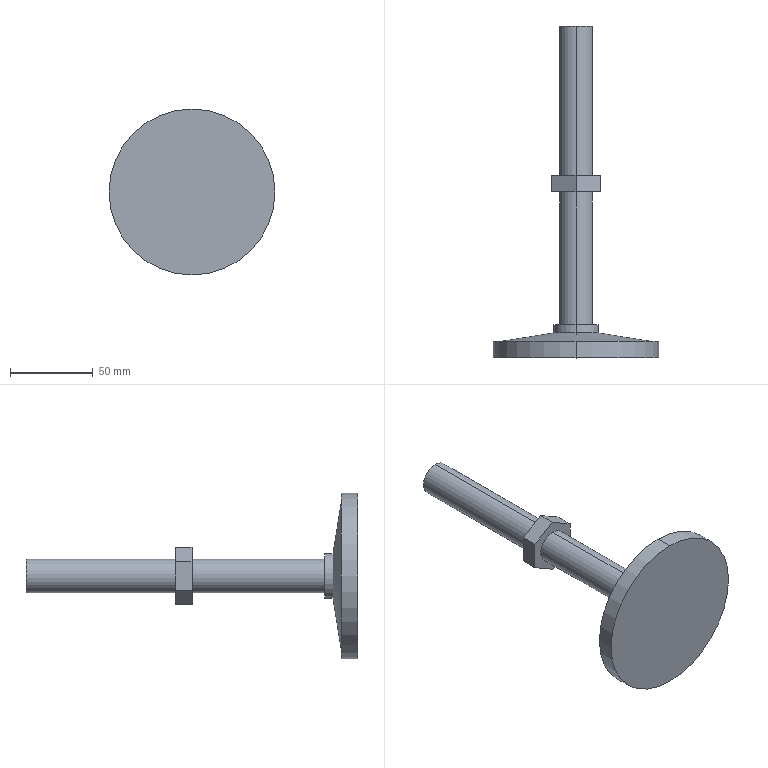Part | SolidWorks | features Boss 1, Revolution 1 | 1 solid | 22 faces | box 100 x 200 x 100 mm | volume 157266 mm3 | plane 12 | cylinder 8 | cone 2 | commonest cylinder face diameters 20 x4 26.809 x2 100 x2
STEP:
#1=CARTESIAN_POINT('',(0.,200.,-10.));
#2=VERTEX_POINT('',#1);
#3=CARTESIAN_POINT('',(0.,200.,10.));
#4=VERTEX_POINT('',#3);
#5=CARTESIAN_POINT('',(0.,200.,0.));
#6=DIRECTION('',(0.,-1.,0.));
#7=DIRECTION('',(0.,0.,-1.));
#8=AXIS2_PLACEMENT_3D('',#5,#6,#7);
#9=CIRCLE('',#8,10.);
#10=EDGE_CURVE('',#2,#4,#9,.T.);
#11=ORIENTED_EDGE('',*,*,#10,.T.);
#12=CARTESIAN_POINT('',(0.,110.,10.));
#13=VERTEX_POINT('',#12);
#14=CARTESIAN_POINT('',(0.,0.,10.));
#15=DIRECTION('',(0.,-1.,0.));
#16=VECTOR('',#15,1000.);
#17=LINE('',#14,#16);
#18=EDGE_CURVE('',#4,#13,#17,.T.);
#19=ORIENTED_EDGE('',*,*,#18,.T.);
#20=CARTESIAN_POINT('',(0.,110.,-10.));
#21=VERTEX_POINT('',#20);
#22=CARTESIAN_POINT('',(0.,110.,0.));
#23=DIRECTION('',(0.,1.,0.));
#24=DIRECTION('',(0.,0.,-1.));
#25=AXIS2_PLACEMENT_3D('',#22,#23,#24);
#26=CIRCLE('',#25,10.);
#27=EDGE_CURVE('',#13,#21,#26,.T.);
#28=ORIENTED_EDGE('',*,*,#27,.T.);
#29=CARTESIAN_POINT('',(0.,0.,-10.));
#30=DIRECTION('',(0.,-1.,0.));
#31=VECTOR('',#30,1000.);
#32=LINE('',#29,#31);
#33=EDGE_CURVE('',#2,#21,#32,.T.);
#34=ORIENTED_EDGE('',*,*,#33,.F.);
#35=EDGE_LOOP('',(#11,#19,#28,#34));
#36=FACE_OUTER_BOUND('',#35,.T.);
#37=CARTESIAN_POINT('',(0.,0.,0.));
#38=DIRECTION('',(0.,-1.,0.));
#39=DIRECTION('',(0.,0.,-1.));
#40=AXIS2_PLACEMENT_3D('',#37,#38,#39);
#41=CYLINDRICAL_SURFACE('',#40,10.);
#42=ADVANCED_FACE('',(#36),#41,.T.);
#43=CARTESIAN_POINT('',(0.,100.,10.));
#44=VERTEX_POINT('',#43);
#45=CARTESIAN_POINT('',(0.,100.,-10.));
#46=VERTEX_POINT('',#45);
#47=CARTESIAN_POINT('',(0.,100.,0.));
#48=DIRECTION('',(0.,1.,0.));
#49=DIRECTION('',(0.,0.,-1.));
#50=AXIS2_PLACEMENT_3D('',#47,#48,#49);
#51=CIRCLE('',#50,10.);
#52=EDGE_CURVE('',#44,#46,#51,.T.);
#53=ORIENTED_EDGE('',*,*,#52,.F.);
#54=CARTESIAN_POINT('',(0.,20.,10.));
#55=VERTEX_POINT('',#54);
#56=CARTESIAN_POINT('',(0.,0.,10.));
#57=DIRECTION('',(0.,-1.,0.));
#58=VECTOR('',#57,1000.);
#59=LINE('',#56,#58);
#60=EDGE_CURVE('',#44,#55,#59,.T.);
#61=ORIENTED_EDGE('',*,*,#60,.T.);
#62=CARTESIAN_POINT('',(0.,20.,-10.));
#63=VERTEX_POINT('',#62);
#64=CARTESIAN_POINT('',(0.,20.,0.));
#65=DIRECTION('',(0.,-1.,0.));
#66=DIRECTION('',(0.,0.,-1.));
#67=AXIS2_PLACEMENT_3D('',#64,#65,#66);
#68=CIRCLE('',#67,10.);
#69=EDGE_CURVE('',#63,#55,#68,.T.);
#70=ORIENTED_EDGE('',*,*,#69,.F.);
#71=CARTESIAN_POINT('',(0.,0.,-10.));
#72=DIRECTION('',(0.,-1.,0.));
#73=VECTOR('',#72,1000.);
#74=LINE('',#71,#73);
#75=EDGE_CURVE('',#46,#63,#74,.T.);
#76=ORIENTED_EDGE('',*,*,#75,.F.);
#77=EDGE_LOOP('',(#53,#61,#70,#76));
#78=FACE_OUTER_BOUND('',#77,.T.);
#79=CARTESIAN_POINT('',(0.,0.,0.));
#80=DIRECTION('',(0.,-1.,0.));
#81=DIRECTION('',(0.,0.,-1.));
#82=AXIS2_PLACEMENT_3D('',#79,#80,#81);
#83=CYLINDRICAL_SURFACE('',#82,10.);
#84=ADVANCED_FACE('',(#78),#83,.T.);
#85=CARTESIAN_POINT('',(0.,20.,-13.405));
#86=VERTEX_POINT('',#85);
#87=CARTESIAN_POINT('',(0.,20.,13.405));
#88=VERTEX_POINT('',#87);
#89=CARTESIAN_POINT('',(0.,20.,0.));
#90=DIRECTION('',(0.,-1.,0.));
#91=DIRECTION('',(0.,0.,-1.));
#92=AXIS2_PLACEMENT_3D('',#89,#90,#91);
#93=CIRCLE('',#92,13.405);
#94=EDGE_CURVE('',#86,#88,#93,.T.);
#95=ORIENTED_EDGE('',*,*,#94,.T.);
#96=CARTESIAN_POINT('',(0.,15.,13.405));
#97=VERTEX_POINT('',#96);
#98=CARTESIAN_POINT('',(0.,0.,13.405));
#99=DIRECTION('',(0.,-1.,0.));
#100=VECTOR('',#99,1000.);
#101=LINE('',#98,#100);
#102=EDGE_CURVE('',#88,#97,#101,.T.);
#103=ORIENTED_EDGE('',*,*,#102,.T.);
#104=CARTESIAN_POINT('',(0.,15.,-13.405));
#105=VERTEX_POINT('',#104);
#106=CARTESIAN_POINT('',(0.,15.,0.));
#107=DIRECTION('',(0.,-1.,0.));
#108=DIRECTION('',(0.,0.,-1.));
#109=AXIS2_PLACEMENT_3D('',#106,#107,#108);
#110=CIRCLE('',#109,13.405);
#111=EDGE_CURVE('',#105,#97,#110,.T.);
#112=ORIENTED_EDGE('',*,*,#111,.F.);
#113=CARTESIAN_POINT('',(0.,0.,-13.405));
#114=DIRECTION('',(0.,-1.,0.));
#115=VECTOR('',#114,1000.);
#116=LINE('',#113,#115);
#117=EDGE_CURVE('',#86,#105,#116,.T.);
#118=ORIENTED_EDGE('',*,*,#117,.F.);
#119=EDGE_LOOP('',(#95,#103,#112,#118));
#120=FACE_OUTER_BOUND('',#119,.T.);
#121=CARTESIAN_POINT('',(0.,0.,0.));
#122=DIRECTION('',(0.,-1.,0.));
#123=DIRECTION('',(0.,0.,-1.));
#124=AXIS2_PLACEMENT_3D('',#121,#122,#123);
#125=CYLINDRICAL_SURFACE('',#124,13.405);
#126=ADVANCED_FACE('',(#120),#125,.T.);
#127=ORIENTED_EDGE('',*,*,#111,.T.);
#128=CARTESIAN_POINT('',(0.,10.,45.));
#129=VERTEX_POINT('',#128);
#130=CARTESIAN_POINT('',(0.,10.,45.));
#131=DIRECTION('',(0.,-0.1563,0.9877));
#132=VECTOR('',#131,1000.);
#133=LINE('',#130,#132);
#134=EDGE_CURVE('',#97,#129,#133,.T.);
#135=ORIENTED_EDGE('',*,*,#134,.T.);
#136=CARTESIAN_POINT('',(0.,10.,-45.));
#137=VERTEX_POINT('',#136);
#138=CARTESIAN_POINT('',(0.,10.,0.));
#139=DIRECTION('',(0.,-1.,0.));
#140=DIRECTION('',(0.,0.,-1.));
#141=AXIS2_PLACEMENT_3D('',#138,#139,#140);
#142=CIRCLE('',#141,45.);
#143=EDGE_CURVE('',#137,#129,#142,.T.);
#144=ORIENTED_EDGE('',*,*,#143,.F.);
#145=CARTESIAN_POINT('',(0.,10.,-45.));
#146=DIRECTION('',(0.,-0.1563,-0.9877));
#147=VECTOR('',#146,1000.);
#148=LINE('',#145,#147);
#149=EDGE_CURVE('',#105,#137,#148,.T.);
#150=ORIENTED_EDGE('',*,*,#149,.F.);
#151=EDGE_LOOP('',(#127,#135,#144,#150));
#152=FACE_OUTER_BOUND('',#151,.T.);
#153=CARTESIAN_POINT('',(0.,10.,0.));
#154=DIRECTION('',(0.,-1.,0.));
#155=DIRECTION('',(0.,0.,-1.));
#156=AXIS2_PLACEMENT_3D('',#153,#154,#155);
#157=CONICAL_SURFACE('',#156,45.,1.414);
#158=ADVANCED_FACE('',(#152),#157,.T.);
#159=CARTESIAN_POINT('',(0.,10.,-50.));
#160=VERTEX_POINT('',#159);
#161=CARTESIAN_POINT('',(0.,10.,50.));
#162=VERTEX_POINT('',#161);
#163=CARTESIAN_POINT('',(0.,10.,0.));
#164=DIRECTION('',(0.,-1.,0.));
#165=DIRECTION('',(0.,0.,-1.));
#166=AXIS2_PLACEMENT_3D('',#163,#164,#165);
#167=CIRCLE('',#166,50.);
#168=EDGE_CURVE('',#160,#162,#167,.T.);
#169=ORIENTED_EDGE('',*,*,#168,.T.);
#170=CARTESIAN_POINT('',(0.,0.,50.));
#171=VERTEX_POINT('',#170);
#172=CARTESIAN_POINT('',(0.,0.,50.));
#173=DIRECTION('',(0.,-1.,0.));
#174=VECTOR('',#173,1000.);
#175=LINE('',#172,#174);
#176=EDGE_CURVE('',#162,#171,#175,.T.);
#177=ORIENTED_EDGE('',*,*,#176,.T.);
#178=CARTESIAN_POINT('',(0.,0.,-50.));
#179=VERTEX_POINT('',#178);
#180=CARTESIAN_POINT('',(0.,0.,0.));
#181=DIRECTION('',(0.,-1.,0.));
#182=DIRECTION('',(0.,0.,-1.));
#183=AXIS2_PLACEMENT_3D('',#180,#181,#182);
#184=CIRCLE('',#183,50.);
#185=EDGE_CURVE('',#179,#171,#184,.T.);
#186=ORIENTED_EDGE('',*,*,#185,.F.);
#187=CARTESIAN_POINT('',(0.,0.,-50.));
#188=DIRECTION('',(0.,-1.,0.));
#189=VECTOR('',#188,1000.);
#190=LINE('',#187,#189);
#191=EDGE_CURVE('',#160,#179,#190,.T.);
#192=ORIENTED_EDGE('',*,*,#191,.F.);
#193=EDGE_LOOP('',(#169,#177,#186,#192));
#194=FACE_OUTER_BOUND('',#193,.T.);
#195=CARTESIAN_POINT('',(0.,0.,0.));
#196=DIRECTION('',(0.,-1.,0.));
#197=DIRECTION('',(0.,0.,-1.));
#198=AXIS2_PLACEMENT_3D('',#195,#196,#197);
#199=CYLINDRICAL_SURFACE('',#198,50.);
#200=ADVANCED_FACE('',(#194),#199,.T.);
#201=ORIENTED_EDGE('',*,*,#185,.T.);
#202=CARTESIAN_POINT('',(0.,0.,0.));
#203=DIRECTION('',(0.,-1.,0.));
#204=DIRECTION('',(0.,0.,-1.));
#205=AXIS2_PLACEMENT_3D('',#202,#203,#204);
#206=CIRCLE('',#205,50.);
#207=EDGE_CURVE('',#171,#179,#206,.T.);
#208=ORIENTED_EDGE('',*,*,#207,.T.);
#209=EDGE_LOOP('',(#201,#208));
#210=FACE_OUTER_BOUND('',#209,.T.);
#211=CARTESIAN_POINT('',(0.,0.,0.));
#212=DIRECTION('',(0.,-1.,0.));
#213=DIRECTION('',(0.,0.,-1.));
#214=AXIS2_PLACEMENT_3D('',#211,#212,#213);
#215=PLANE('',#214);
#216=ADVANCED_FACE('',(#210),#215,.T.);
#217=ORIENTED_EDGE('',*,*,#176,.F.);
#218=CARTESIAN_POINT('',(0.,10.,0.));
#219=DIRECTION('',(0.,-1.,0.));
#220=DIRECTION('',(0.,0.,-1.));
#221=AXIS2_PLACEMENT_3D('',#218,#219,#220);
#222=CIRCLE('',#221,50.);
#223=EDGE_CURVE('',#162,#160,#222,.T.);
#224=ORIENTED_EDGE('',*,*,#223,.T.);
#225=ORIENTED_EDGE('',*,*,#191,.T.);
#226=ORIENTED_EDGE('',*,*,#207,.F.);
#227=EDGE_LOOP('',(#217,#224,#225,#226));
#228=FACE_OUTER_BOUND('',#227,.T.);
#229=CARTESIAN_POINT('',(0.,0.,0.));
#230=DIRECTION('',(0.,-1.,0.));
#231=DIRECTION('',(0.,0.,-1.));
#232=AXIS2_PLACEMENT_3D('',#229,#230,#231);
#233=CYLINDRICAL_SURFACE('',#232,50.);
#234=ADVANCED_FACE('',(#228),#233,.T.);
#235=ORIENTED_EDGE('',*,*,#143,.T.);
#236=CARTESIAN_POINT('',(0.,10.,0.));
#237=DIRECTION('',(0.,-1.,0.));
#238=DIRECTION('',(0.,0.,-1.));
#239=AXIS2_PLACEMENT_3D('',#236,#237,#238);
#240=CIRCLE('',#239,45.);
#241=EDGE_CURVE('',#129,#137,#240,.T.);
#242=ORIENTED_EDGE('',*,*,#241,.T.);
#243=EDGE_LOOP('',(#235,#242));
#244=FACE_BOUND('',#243,.T.);
#245=ORIENTED_EDGE('',*,*,#168,.F.);
#246=ORIENTED_EDGE('',*,*,#223,.F.);
#247=EDGE_LOOP('',(#245,#246));
#248=FACE_OUTER_BOUND('',#247,.T.);
#249=CARTESIAN_POINT('',(50.,10.,0.));
#250=DIRECTION('',(0.,1.,0.));
#251=DIRECTION('',(0.,0.,1.));
#252=AXIS2_PLACEMENT_3D('',#249,#250,#251);
#253=PLANE('',#252);
#254=ADVANCED_FACE('',(#244,#248),#253,.T.);
#255=ORIENTED_EDGE('',*,*,#134,.F.);
#256=CARTESIAN_POINT('',(0.,15.,0.));
#257=DIRECTION('',(0.,-1.,0.));
#258=DIRECTION('',(0.,0.,-1.));
#259=AXIS2_PLACEMENT_3D('',#256,#257,#258);
#260=CIRCLE('',#259,13.405);
#261=EDGE_CURVE('',#97,#105,#260,.T.);
#262=ORIENTED_EDGE('',*,*,#261,.T.);
#263=ORIENTED_EDGE('',*,*,#149,.T.);
#264=ORIENTED_EDGE('',*,*,#241,.F.);
#265=EDGE_LOOP('',(#255,#262,#263,#264));
#266=FACE_OUTER_BOUND('',#265,.T.);
#267=CARTESIAN_POINT('',(0.,10.,0.));
#268=DIRECTION('',(0.,-1.,0.));
#269=DIRECTION('',(0.,0.,-1.));
#270=AXIS2_PLACEMENT_3D('',#267,#268,#269);
#271=CONICAL_SURFACE('',#270,45.,1.414);
#272=ADVANCED_FACE('',(#266),#271,.T.);
#273=ORIENTED_EDGE('',*,*,#102,.F.);
#274=CARTESIAN_POINT('',(0.,20.,0.));
#275=DIRECTION('',(0.,-1.,0.));
#276=DIRECTION('',(0.,0.,-1.));
#277=AXIS2_PLACEMENT_3D('',#274,#275,#276);
#278=CIRCLE('',#277,13.405);
#279=EDGE_CURVE('',#88,#86,#278,.T.);
#280=ORIENTED_EDGE('',*,*,#279,.T.);
#281=ORIENTED_EDGE('',*,*,#117,.T.);
#282=ORIENTED_EDGE('',*,*,#261,.F.);
#283=EDGE_LOOP('',(#273,#280,#281,#282));
#284=FACE_OUTER_BOUND('',#283,.T.);
#285=CARTESIAN_POINT('',(0.,0.,0.));
#286=DIRECTION('',(0.,-1.,0.));
#287=DIRECTION('',(0.,0.,-1.));
#288=AXIS2_PLACEMENT_3D('',#285,#286,#287);
#289=CYLINDRICAL_SURFACE('',#288,13.405);
#290=ADVANCED_FACE('',(#284),#289,.T.);
#291=ORIENTED_EDGE('',*,*,#69,.T.);
#292=CARTESIAN_POINT('',(0.,20.,0.));
#293=DIRECTION('',(0.,-1.,0.));
#294=DIRECTION('',(0.,0.,-1.));
#295=AXIS2_PLACEMENT_3D('',#292,#293,#294);
#296=CIRCLE('',#295,10.);
#297=EDGE_CURVE('',#55,#63,#296,.T.);
#298=ORIENTED_EDGE('',*,*,#297,.T.);
#299=EDGE_LOOP('',(#291,#298));
#300=FACE_BOUND('',#299,.T.);
#301=ORIENTED_EDGE('',*,*,#94,.F.);
#302=ORIENTED_EDGE('',*,*,#279,.F.);
#303=EDGE_LOOP('',(#301,#302));
#304=FACE_OUTER_BOUND('',#303,.T.);
#305=CARTESIAN_POINT('',(13.405,20.,0.));
#306=DIRECTION('',(0.,1.,0.));
#307=DIRECTION('',(0.,0.,1.));
#308=AXIS2_PLACEMENT_3D('',#305,#306,#307);
#309=PLANE('',#308);
#310=ADVANCED_FACE('',(#300,#304),#309,.T.);
#311=ORIENTED_EDGE('',*,*,#60,.F.);
#312=CARTESIAN_POINT('',(0.,100.,0.));
#313=DIRECTION('',(0.,1.,0.));
#314=DIRECTION('',(0.,0.,-1.));
#315=AXIS2_PLACEMENT_3D('',#312,#313,#314);
#316=CIRCLE('',#315,10.);
#317=EDGE_CURVE('',#46,#44,#316,.T.);
#318=ORIENTED_EDGE('',*,*,#317,.F.);
#319=ORIENTED_EDGE('',*,*,#75,.T.);
#320=ORIENTED_EDGE('',*,*,#297,.F.);
#321=EDGE_LOOP('',(#311,#318,#319,#320));
#322=FACE_OUTER_BOUND('',#321,.T.);
#323=CARTESIAN_POINT('',(0.,0.,0.));
#324=DIRECTION('',(0.,-1.,0.));
#325=DIRECTION('',(0.,0.,-1.));
#326=AXIS2_PLACEMENT_3D('',#323,#324,#325);
#327=CYLINDRICAL_SURFACE('',#326,10.);
#328=ADVANCED_FACE('',(#322),#327,.T.);
#329=CARTESIAN_POINT('',(15.,110.,-8.66));
#330=VERTEX_POINT('',#329);
#331=CARTESIAN_POINT('',(15.,110.,8.66));
#332=VERTEX_POINT('',#331);
#333=CARTESIAN_POINT('',(15.,110.,-35.785));
#334=DIRECTION('',(0.,0.,1.));
#335=VECTOR('',#334,1000.);
#336=LINE('',#333,#335);
#337=EDGE_CURVE('',#330,#332,#336,.T.);
#338=ORIENTED_EDGE('',*,*,#337,.T.);
#339=CARTESIAN_POINT('',(15.,100.,8.66));
#340=VERTEX_POINT('',#339);
#341=CARTESIAN_POINT('',(15.,100.,8.66));
#342=DIRECTION('',(0.,1.,0.));
#343=VECTOR('',#342,1000.);
#344=LINE('',#341,#343);
#345=EDGE_CURVE('',#340,#332,#344,.T.);
#346=ORIENTED_EDGE('',*,*,#345,.F.);
#347=CARTESIAN_POINT('',(15.,100.,-8.66));
#348=VERTEX_POINT('',#347);
#349=CARTESIAN_POINT('',(15.,100.,-35.785));
#350=DIRECTION('',(0.,0.,1.));
#351=VECTOR('',#350,1000.);
#352=LINE('',#349,#351);
#353=EDGE_CURVE('',#348,#340,#352,.T.);
#354=ORIENTED_EDGE('',*,*,#353,.F.);
#355=CARTESIAN_POINT('',(15.,100.,-8.66));
#356=DIRECTION('',(0.,1.,0.));
#357=VECTOR('',#356,1000.);
#358=LINE('',#355,#357);
#359=EDGE_CURVE('',#348,#330,#358,.T.);
#360=ORIENTED_EDGE('',*,*,#359,.T.);
#361=EDGE_LOOP('',(#338,#346,#354,#360));
#362=FACE_OUTER_BOUND('',#361,.T.);
#363=CARTESIAN_POINT('',(15.,100.,-35.785));
#364=DIRECTION('',(-1.,0.,0.));
#365=DIRECTION('',(0.,0.,1.));
#366=AXIS2_PLACEMENT_3D('',#363,#364,#365);
#367=PLANE('',#366);
#368=ADVANCED_FACE('',(#362),#367,.F.);
#369=CARTESIAN_POINT('',(0.,110.,17.321));
#370=VERTEX_POINT('',#369);
#371=CARTESIAN_POINT('',(22.996,110.,4.044));
#372=DIRECTION('',(-0.866,0.,0.5));
#373=VECTOR('',#372,1000.);
#374=LINE('',#371,#373);
#375=EDGE_CURVE('',#332,#370,#374,.T.);
#376=ORIENTED_EDGE('',*,*,#375,.T.);
#377=CARTESIAN_POINT('',(0.,100.,17.321));
#378=VERTEX_POINT('',#377);
#379=CARTESIAN_POINT('',(0.,100.,17.321));
#380=DIRECTION('',(0.,1.,0.));
#381=VECTOR('',#380,1000.);
#382=LINE('',#379,#381);
#383=EDGE_CURVE('',#378,#370,#382,.T.);
#384=ORIENTED_EDGE('',*,*,#383,.F.);
#385=CARTESIAN_POINT('',(22.996,100.,4.044));
#386=DIRECTION('',(-0.866,0.,0.5));
#387=VECTOR('',#386,1000.);
#388=LINE('',#385,#387);
#389=EDGE_CURVE('',#340,#378,#388,.T.);
#390=ORIENTED_EDGE('',*,*,#389,.F.);
#391=ORIENTED_EDGE('',*,*,#345,.T.);
#392=EDGE_LOOP('',(#376,#384,#390,#391));
#393=FACE_OUTER_BOUND('',#392,.T.);
#394=CARTESIAN_POINT('',(22.996,100.,4.044));
#395=DIRECTION('',(-0.5,0.,-0.866));
#396=DIRECTION('',(-0.866,0.,0.5));
#397=AXIS2_PLACEMENT_3D('',#394,#395,#396);
#398=PLANE('',#397);
#399=ADVANCED_FACE('',(#393),#398,.F.);
#400=CARTESIAN_POINT('',(-15.,110.,8.66));
#401=VERTEX_POINT('',#400);
#402=CARTESIAN_POINT('',(-22.996,110.,4.044));
#403=DIRECTION('',(-0.866,0.,-0.5));
#404=VECTOR('',#403,1000.);
#405=LINE('',#402,#404);
#406=EDGE_CURVE('',#370,#401,#405,.T.);
#407=ORIENTED_EDGE('',*,*,#406,.T.);
#408=CARTESIAN_POINT('',(-15.,100.,8.66));
#409=VERTEX_POINT('',#408);
#410=CARTESIAN_POINT('',(-15.,100.,8.66));
#411=DIRECTION('',(0.,1.,0.));
#412=VECTOR('',#411,1000.);
#413=LINE('',#410,#412);
#414=EDGE_CURVE('',#409,#401,#413,.T.);
#415=ORIENTED_EDGE('',*,*,#414,.F.);
#416=CARTESIAN_POINT('',(-22.996,100.,4.044));
#417=DIRECTION('',(-0.866,0.,-0.5));
#418=VECTOR('',#417,1000.);
#419=LINE('',#416,#418);
#420=EDGE_CURVE('',#378,#409,#419,.T.);
#421=ORIENTED_EDGE('',*,*,#420,.F.);
#422=ORIENTED_EDGE('',*,*,#383,.T.);
#423=EDGE_LOOP('',(#407,#415,#421,#422));
#424=FACE_OUTER_BOUND('',#423,.T.);
#425=CARTESIAN_POINT('',(-22.996,100.,4.044));
#426=DIRECTION('',(0.5,0.,-0.866));
#427=DIRECTION('',(-0.866,0.,-0.5));
#428=AXIS2_PLACEMENT_3D('',#425,#426,#427);
#429=PLANE('',#428);
#430=ADVANCED_FACE('',(#424),#429,.F.);
#431=CARTESIAN_POINT('',(-15.,110.,-8.66));
#432=VERTEX_POINT('',#431);
#433=CARTESIAN_POINT('',(-15.,110.,-35.785));
#434=DIRECTION('',(0.,0.,-1.));
#435=VECTOR('',#434,1000.);
#436=LINE('',#433,#435);
#437=EDGE_CURVE('',#401,#432,#436,.T.);
#438=ORIENTED_EDGE('',*,*,#437,.T.);
#439=CARTESIAN_POINT('',(-15.,100.,-8.66));
#440=VERTEX_POINT('',#439);
#441=CARTESIAN_POINT('',(-15.,100.,-8.66));
#442=DIRECTION('',(0.,1.,0.));
#443=VECTOR('',#442,1000.);
#444=LINE('',#441,#443);
#445=EDGE_CURVE('',#440,#432,#444,.T.);
#446=ORIENTED_EDGE('',*,*,#445,.F.);
#447=CARTESIAN_POINT('',(-15.,100.,-35.785));
#448=DIRECTION('',(0.,0.,-1.));
#449=VECTOR('',#448,1000.);
#450=LINE('',#447,#449);
#451=EDGE_CURVE('',#409,#440,#450,.T.);
#452=ORIENTED_EDGE('',*,*,#451,.F.);
#453=ORIENTED_EDGE('',*,*,#414,.T.);
#454=EDGE_LOOP('',(#438,#446,#452,#453));
#455=FACE_OUTER_BOUND('',#454,.T.);
#456=CARTESIAN_POINT('',(-15.,100.,-35.785));
#457=DIRECTION('',(1.,0.,0.));
#458=DIRECTION('',(0.,0.,-1.));
#459=AXIS2_PLACEMENT_3D('',#456,#457,#458);
#460=PLANE('',#459);
#461=ADVANCED_FACE('',(#455),#460,.F.);
#462=CARTESIAN_POINT('',(0.,110.,-17.321));
#463=VERTEX_POINT('',#462);
#464=CARTESIAN_POINT('',(7.996,110.,-21.937));
#465=DIRECTION('',(0.866,0.,-0.5));
#466=VECTOR('',#465,1000.);
#467=LINE('',#464,#466);
#468=EDGE_CURVE('',#432,#463,#467,.T.);
#469=ORIENTED_EDGE('',*,*,#468,.T.);
#470=CARTESIAN_POINT('',(0.,100.,-17.321));
#471=VERTEX_POINT('',#470);
#472=CARTESIAN_POINT('',(0.,100.,-17.321));
#473=DIRECTION('',(0.,1.,0.));
#474=VECTOR('',#473,1000.);
#475=LINE('',#472,#474);
#476=EDGE_CURVE('',#471,#463,#475,.T.);
#477=ORIENTED_EDGE('',*,*,#476,.F.);
#478=CARTESIAN_POINT('',(7.996,100.,-21.937));
#479=DIRECTION('',(0.866,0.,-0.5));
#480=VECTOR('',#479,1000.);
#481=LINE('',#478,#480);
#482=EDGE_CURVE('',#440,#471,#481,.T.);
#483=ORIENTED_EDGE('',*,*,#482,.F.);
#484=ORIENTED_EDGE('',*,*,#445,.T.);
#485=EDGE_LOOP('',(#469,#477,#483,#484));
#486=FACE_OUTER_BOUND('',#485,.T.);
#487=CARTESIAN_POINT('',(7.996,100.,-21.937));
#488=DIRECTION('',(0.5,0.,0.866));
#489=DIRECTION('',(0.866,0.,-0.5));
#490=AXIS2_PLACEMENT_3D('',#487,#488,#489);
#491=PLANE('',#490);
#492=ADVANCED_FACE('',(#486),#491,.F.);
#493=CARTESIAN_POINT('',(-7.996,110.,-21.937));
#494=DIRECTION('',(0.866,0.,0.5));
#495=VECTOR('',#494,1000.);
#496=LINE('',#493,#495);
#497=EDGE_CURVE('',#463,#330,#496,.T.);
#498=ORIENTED_EDGE('',*,*,#497,.T.);
#499=ORIENTED_EDGE('',*,*,#359,.F.);
#500=CARTESIAN_POINT('',(-7.996,100.,-21.937));
#501=DIRECTION('',(0.866,0.,0.5));
#502=VECTOR('',#501,1000.);
#503=LINE('',#500,#502);
#504=EDGE_CURVE('',#471,#348,#503,.T.);
#505=ORIENTED_EDGE('',*,*,#504,.F.);
#506=ORIENTED_EDGE('',*,*,#476,.T.);
#507=EDGE_LOOP('',(#498,#499,#505,#506));
#508=FACE_OUTER_BOUND('',#507,.T.);
#509=CARTESIAN_POINT('',(-7.996,100.,-21.937));
#510=DIRECTION('',(-0.5,0.,0.866));
#511=DIRECTION('',(0.866,0.,0.5));
#512=AXIS2_PLACEMENT_3D('',#509,#510,#511);
#513=PLANE('',#512);
#514=ADVANCED_FACE('',(#508),#513,.F.);
#515=ORIENTED_EDGE('',*,*,#317,.T.);
#516=ORIENTED_EDGE('',*,*,#52,.T.);
#517=EDGE_LOOP('',(#515,#516));
#518=FACE_BOUND('',#517,.T.);
#519=ORIENTED_EDGE('',*,*,#353,.T.);
#520=ORIENTED_EDGE('',*,*,#389,.T.);
#521=ORIENTED_EDGE('',*,*,#420,.T.);
#522=ORIENTED_EDGE('',*,*,#451,.T.);
#523=ORIENTED_EDGE('',*,*,#482,.T.);
#524=ORIENTED_EDGE('',*,*,#504,.T.);
#525=EDGE_LOOP('',(#519,#520,#521,#522,#523,#524));
#526=FACE_OUTER_BOUND('',#525,.T.);
#527=CARTESIAN_POINT('',(0.,100.,-35.785));
#528=DIRECTION('',(0.,-1.,0.));
#529=DIRECTION('',(0.,0.,-1.));
#530=AXIS2_PLACEMENT_3D('',#527,#528,#529);
#531=PLANE('',#530);
#532=ADVANCED_FACE('',(#518,#526),#531,.T.);
#533=CARTESIAN_POINT('',(0.,110.,0.));
#534=DIRECTION('',(0.,1.,0.));
#535=DIRECTION('',(0.,0.,-1.));
#536=AXIS2_PLACEMENT_3D('',#533,#534,#535);
#537=CIRCLE('',#536,10.);
#538=EDGE_CURVE('',#21,#13,#537,.T.);
#539=ORIENTED_EDGE('',*,*,#538,.F.);
#540=ORIENTED_EDGE('',*,*,#27,.F.);
#541=EDGE_LOOP('',(#539,#540));
#542=FACE_BOUND('',#541,.T.);
#543=ORIENTED_EDGE('',*,*,#337,.F.);
#544=ORIENTED_EDGE('',*,*,#497,.F.);
#545=ORIENTED_EDGE('',*,*,#468,.F.);
#546=ORIENTED_EDGE('',*,*,#437,.F.);
#547=ORIENTED_EDGE('',*,*,#406,.F.);
#548=ORIENTED_EDGE('',*,*,#375,.F.);
#549=EDGE_LOOP('',(#543,#544,#545,#546,#547,#548));
#550=FACE_OUTER_BOUND('',#549,.T.);
#551=CARTESIAN_POINT('',(0.,110.,-35.785));
#552=DIRECTION('',(0.,-1.,0.));
#553=DIRECTION('',(0.,0.,-1.));
#554=AXIS2_PLACEMENT_3D('',#551,#552,#553);
#555=PLANE('',#554);
#556=ADVANCED_FACE('',(#542,#550),#555,.F.);
#557=ORIENTED_EDGE('',*,*,#10,.F.);
#558=CARTESIAN_POINT('',(0.,200.,0.));
#559=DIRECTION('',(0.,-1.,0.));
#560=DIRECTION('',(0.,0.,-1.));
#561=AXIS2_PLACEMENT_3D('',#558,#559,#560);
#562=CIRCLE('',#561,10.);
#563=EDGE_CURVE('',#4,#2,#562,.T.);
#564=ORIENTED_EDGE('',*,*,#563,.F.);
#565=EDGE_LOOP('',(#557,#564));
#566=FACE_OUTER_BOUND('',#565,.T.);
#567=CARTESIAN_POINT('',(10.,200.,0.));
#568=DIRECTION('',(0.,1.,0.));
#569=DIRECTION('',(0.,0.,1.));
#570=AXIS2_PLACEMENT_3D('',#567,#568,#569);
#571=PLANE('',#570);
#572=ADVANCED_FACE('',(#566),#571,.T.);
#573=ORIENTED_EDGE('',*,*,#18,.F.);
#574=ORIENTED_EDGE('',*,*,#563,.T.);
#575=ORIENTED_EDGE('',*,*,#33,.T.);
#576=ORIENTED_EDGE('',*,*,#538,.T.);
#577=EDGE_LOOP('',(#573,#574,#575,#576));
#578=FACE_OUTER_BOUND('',#577,.T.);
#579=CARTESIAN_POINT('',(0.,0.,0.));
#580=DIRECTION('',(0.,-1.,0.));
#581=DIRECTION('',(0.,0.,-1.));
#582=AXIS2_PLACEMENT_3D('',#579,#580,#581);
#583=CYLINDRICAL_SURFACE('',#582,10.);
#584=ADVANCED_FACE('',(#578),#583,.T.);
#585=CLOSED_SHELL('',(#42,#84,#126,#158,#200,#216,#234,#254,#272,#290,#310,#328,#368,#399,#430,#461,#492,#514,#532,#556,#572,#584));
#586=MANIFOLD_SOLID_BREP('',#585);
#587=CARTESIAN_POINT('',(0.,0.,0.));
#588=DIRECTION('',(0.,0.,1.));
#589=DIRECTION('',(1.,0.,0.));
#590=AXIS2_PLACEMENT_3D('',#587,#588,#589);
#591=(LENGTH_UNIT()NAMED_UNIT(*)SI_UNIT(.MILLI.,.METRE.));
#592=UNCERTAINTY_MEASURE_WITH_UNIT(LENGTH_MEASURE(0.00001),#591,'','');
#593=(NAMED_UNIT(*)PLANE_ANGLE_UNIT()SI_UNIT($,.RADIAN.));
#594=(NAMED_UNIT(*)SI_UNIT($,.STERADIAN.)SOLID_ANGLE_UNIT());
#595=(GEOMETRIC_REPRESENTATION_CONTEXT(3)GLOBAL_UNCERTAINTY_ASSIGNED_CONTEXT((#592))GLOBAL_UNIT_ASSIGNED_CONTEXT((#591,#593,#594))REPRESENTATION_CONTEXT('',''));
#596=ADVANCED_BREP_SHAPE_REPRESENTATION('',(#586,#590),#595);